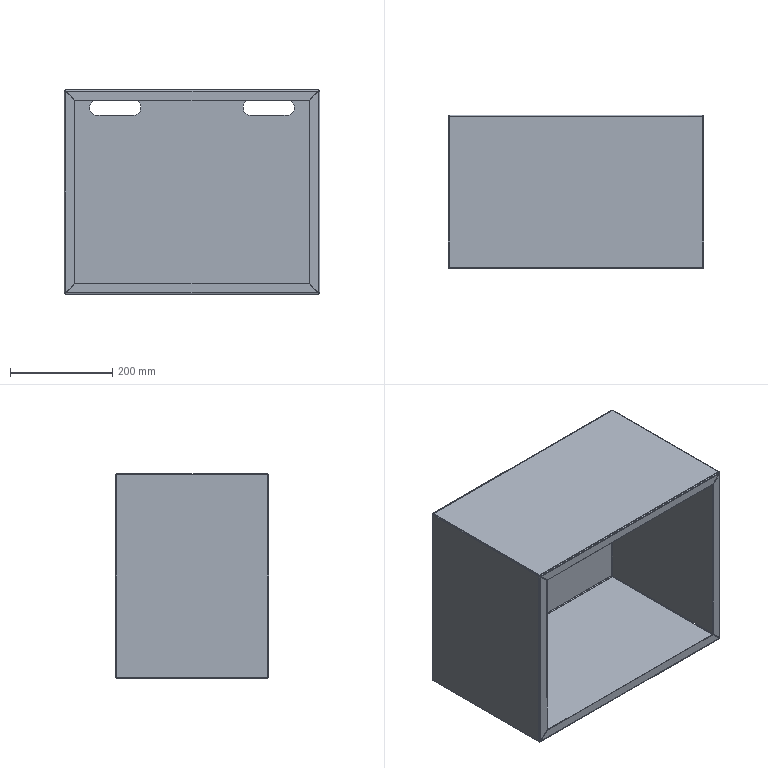Part | STEP file | JBJ-P-1013-07 | 1 solid | 86 faces | box 500 x 300 x 400 mm | volume 907808 mm3 | plane 46 | cylinder 24 | spline 16 | commonest cylinder face diameters 3 x8 5.4 x8 28 x8